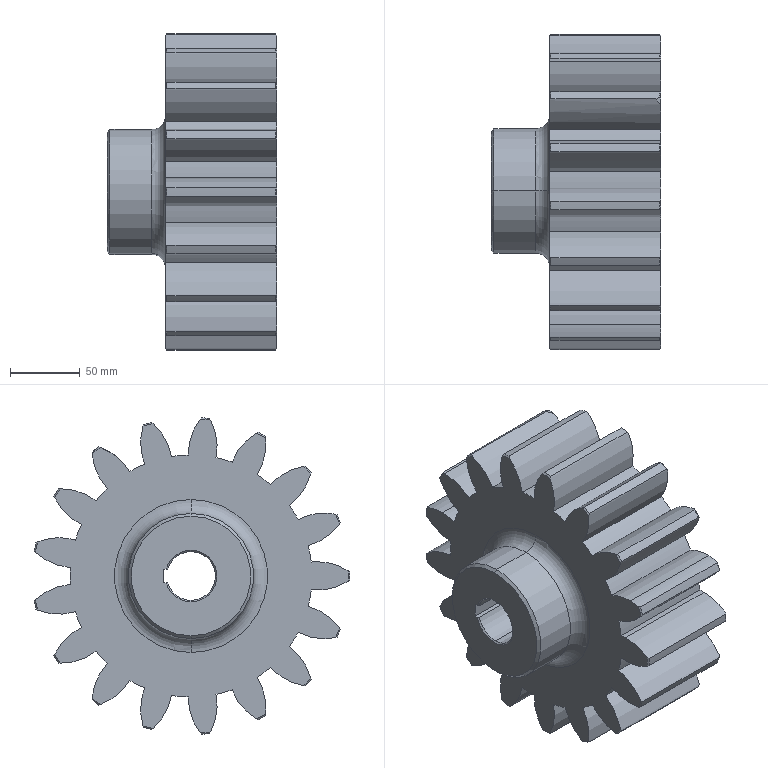Part | SolidWorks | features Chamfer 4, ICE 2, Fillet 1, MoveFace 1, SketchHole 1, Stock 1 | 1 solid | 133 faces | box 122 x 226.585 x 227.513 mm | volume 2321218 mm3 | cylinder 79 | cone 44 | plane 7 | torus 2 | spline 1 | commonest cylinder face diameters 81.6 x38 173.998 x17 228 x17 35 x3 90 x2 100 x2